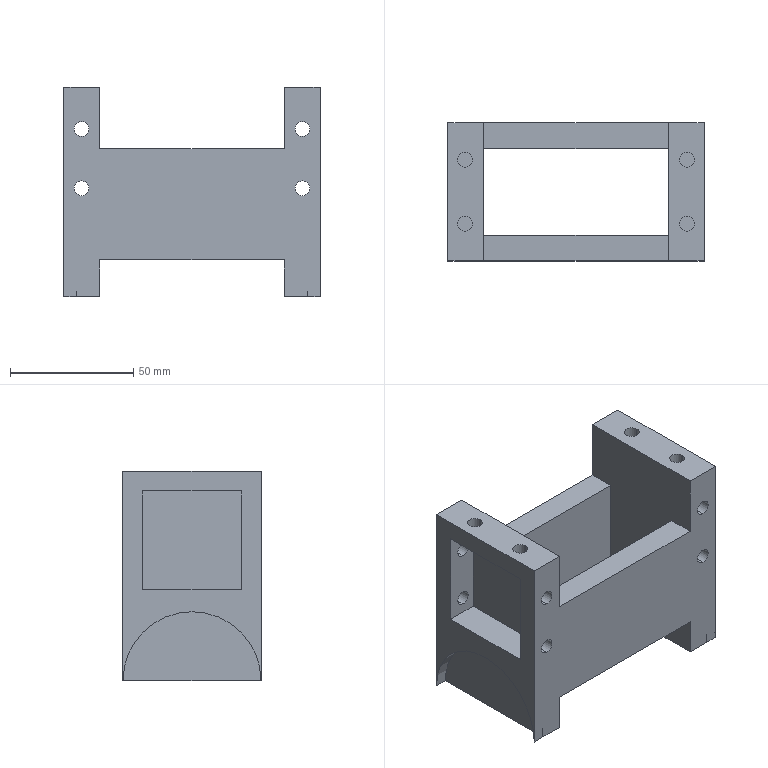Part | STEP file | Cable Carrier Part 1 | 1 solid | 54 faces | box 104 x 56 x 85 mm | volume 152286 mm3 | plane 28 | cylinder 26 | commonest cylinder face diameters 6 x24 56 x2